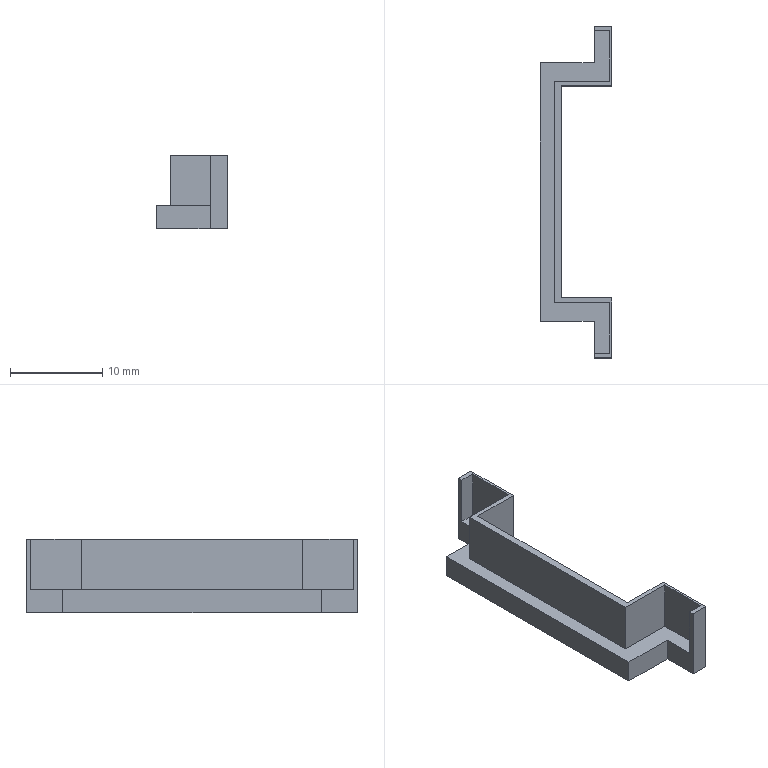Part | STEP file | [DIN35-7.5CA]-1 | 1 solid | 22 faces | box 7.75 x 36 x 8 mm | volume 428.275 mm3 | plane 22
STEP:
#1=CARTESIAN_POINT('',(24.597,-0.5,537.277));
#2=VERTEX_POINT('',#1);
#3=CARTESIAN_POINT('',(24.597,-0.5,539.777));
#4=VERTEX_POINT('',#3);
#5=CARTESIAN_POINT('',(24.597,-0.5,541.277));
#6=DIRECTION('',(0.,0.,1.));
#7=VECTOR('',#6,1000.);
#8=LINE('',#5,#7);
#9=EDGE_CURVE('',#2,#4,#8,.T.);
#10=ORIENTED_EDGE('',*,*,#9,.T.);
#11=CARTESIAN_POINT('',(24.597,27.5,539.777));
#12=VERTEX_POINT('',#11);
#13=CARTESIAN_POINT('',(24.597,-4.,539.777));
#14=DIRECTION('',(0.,1.,0.));
#15=VECTOR('',#14,1000.);
#16=LINE('',#13,#15);
#17=EDGE_CURVE('',#4,#12,#16,.T.);
#18=ORIENTED_EDGE('',*,*,#17,.T.);
#19=CARTESIAN_POINT('',(24.597,27.5,537.277));
#20=VERTEX_POINT('',#19);
#21=CARTESIAN_POINT('',(24.597,27.5,541.277));
#22=DIRECTION('',(0.,0.,-1.));
#23=VECTOR('',#22,1000.);
#24=LINE('',#21,#23);
#25=EDGE_CURVE('',#12,#20,#24,.T.);
#26=ORIENTED_EDGE('',*,*,#25,.T.);
#27=CARTESIAN_POINT('',(24.597,-0.5,537.277));
#28=DIRECTION('',(0.,1.,0.));
#29=VECTOR('',#28,1000.);
#30=LINE('',#27,#29);
#31=EDGE_CURVE('',#2,#20,#30,.T.);
#32=ORIENTED_EDGE('',*,*,#31,.F.);
#33=EDGE_LOOP('',(#10,#18,#26,#32));
#34=FACE_OUTER_BOUND('',#33,.T.);
#35=CARTESIAN_POINT('',(24.597,-0.5,541.277));
#36=DIRECTION('',(-1.,0.,0.));
#37=DIRECTION('',(0.,1.,0.));
#38=AXIS2_PLACEMENT_3D('',#35,#36,#37);
#39=PLANE('',#38);
#40=ADVANCED_FACE('',(#34),#39,.T.);
#41=CARTESIAN_POINT('',(32.347,31.5,545.277));
#42=VERTEX_POINT('',#41);
#43=CARTESIAN_POINT('',(30.447,31.5,545.277));
#44=VERTEX_POINT('',#43);
#45=CARTESIAN_POINT('',(31.397,31.5,545.277));
#46=DIRECTION('',(-1.,0.,0.));
#47=VECTOR('',#46,1000.);
#48=LINE('',#45,#47);
#49=EDGE_CURVE('',#42,#44,#48,.T.);
#50=ORIENTED_EDGE('',*,*,#49,.F.);
#51=CARTESIAN_POINT('',(32.347,31.5,537.277));
#52=VERTEX_POINT('',#51);
#53=CARTESIAN_POINT('',(32.347,31.5,541.277));
#54=DIRECTION('',(0.,0.,1.));
#55=VECTOR('',#54,1000.);
#56=LINE('',#53,#55);
#57=EDGE_CURVE('',#52,#42,#56,.T.);
#58=ORIENTED_EDGE('',*,*,#57,.F.);
#59=CARTESIAN_POINT('',(30.447,31.5,537.277));
#60=VERTEX_POINT('',#59);
#61=CARTESIAN_POINT('',(31.397,31.5,537.277));
#62=DIRECTION('',(1.,0.,0.));
#63=VECTOR('',#62,1000.);
#64=LINE('',#61,#63);
#65=EDGE_CURVE('',#60,#52,#64,.T.);
#66=ORIENTED_EDGE('',*,*,#65,.F.);
#67=CARTESIAN_POINT('',(30.447,31.5,541.277));
#68=DIRECTION('',(0.,0.,-1.));
#69=VECTOR('',#68,1000.);
#70=LINE('',#67,#69);
#71=EDGE_CURVE('',#44,#60,#70,.T.);
#72=ORIENTED_EDGE('',*,*,#71,.F.);
#73=EDGE_LOOP('',(#50,#58,#66,#72));
#74=FACE_OUTER_BOUND('',#73,.T.);
#75=CARTESIAN_POINT('',(31.397,31.5,541.277));
#76=DIRECTION('',(0.,1.,0.));
#77=DIRECTION('',(1.,0.,0.));
#78=AXIS2_PLACEMENT_3D('',#75,#76,#77);
#79=PLANE('',#78);
#80=ADVANCED_FACE('',(#74),#79,.T.);
#81=CARTESIAN_POINT('',(30.447,-4.,545.277));
#82=VERTEX_POINT('',#81);
#83=CARTESIAN_POINT('',(32.097,-4.,545.277));
#84=VERTEX_POINT('',#83);
#85=CARTESIAN_POINT('',(31.347,-4.,545.277));
#86=DIRECTION('',(1.,0.,0.));
#87=VECTOR('',#86,1000.);
#88=LINE('',#85,#87);
#89=EDGE_CURVE('',#82,#84,#88,.T.);
#90=ORIENTED_EDGE('',*,*,#89,.F.);
#91=CARTESIAN_POINT('',(30.447,-4.5,545.277));
#92=VERTEX_POINT('',#91);
#93=CARTESIAN_POINT('',(30.447,-4.5,545.277));
#94=DIRECTION('',(0.,1.,0.));
#95=VECTOR('',#94,1000.);
#96=LINE('',#93,#95);
#97=EDGE_CURVE('',#92,#82,#96,.T.);
#98=ORIENTED_EDGE('',*,*,#97,.F.);
#99=CARTESIAN_POINT('',(32.347,-4.5,545.277));
#100=VERTEX_POINT('',#99);
#101=CARTESIAN_POINT('',(31.397,-4.5,545.277));
#102=DIRECTION('',(1.,0.,0.));
#103=VECTOR('',#102,1000.);
#104=LINE('',#101,#103);
#105=EDGE_CURVE('',#92,#100,#104,.T.);
#106=ORIENTED_EDGE('',*,*,#105,.T.);
#107=CARTESIAN_POINT('',(32.347,2.,545.277));
#108=VERTEX_POINT('',#107);
#109=CARTESIAN_POINT('',(32.347,-4.5,545.277));
#110=DIRECTION('',(0.,1.,0.));
#111=VECTOR('',#110,1000.);
#112=LINE('',#109,#111);
#113=EDGE_CURVE('',#100,#108,#112,.T.);
#114=ORIENTED_EDGE('',*,*,#113,.T.);
#115=CARTESIAN_POINT('',(26.897,2.,545.277));
#116=VERTEX_POINT('',#115);
#117=CARTESIAN_POINT('',(29.622,2.,545.277));
#118=DIRECTION('',(1.,0.,0.));
#119=VECTOR('',#118,1000.);
#120=LINE('',#117,#119);
#121=EDGE_CURVE('',#116,#108,#120,.T.);
#122=ORIENTED_EDGE('',*,*,#121,.F.);
#123=CARTESIAN_POINT('',(26.897,25.,545.277));
#124=VERTEX_POINT('',#123);
#125=CARTESIAN_POINT('',(26.897,2.,545.277));
#126=DIRECTION('',(0.,1.,0.));
#127=VECTOR('',#126,1000.);
#128=LINE('',#125,#127);
#129=EDGE_CURVE('',#116,#124,#128,.T.);
#130=ORIENTED_EDGE('',*,*,#129,.T.);
#131=CARTESIAN_POINT('',(32.347,25.,545.277));
#132=VERTEX_POINT('',#131);
#133=CARTESIAN_POINT('',(29.622,25.,545.277));
#134=DIRECTION('',(-1.,0.,0.));
#135=VECTOR('',#134,1000.);
#136=LINE('',#133,#135);
#137=EDGE_CURVE('',#132,#124,#136,.T.);
#138=ORIENTED_EDGE('',*,*,#137,.F.);
#139=CARTESIAN_POINT('',(32.347,27.5,545.277));
#140=DIRECTION('',(0.,1.,0.));
#141=VECTOR('',#140,1000.);
#142=LINE('',#139,#141);
#143=EDGE_CURVE('',#132,#42,#142,.T.);
#144=ORIENTED_EDGE('',*,*,#143,.T.);
#145=ORIENTED_EDGE('',*,*,#49,.T.);
#146=CARTESIAN_POINT('',(30.447,31.,545.277));
#147=VERTEX_POINT('',#146);
#148=CARTESIAN_POINT('',(30.447,27.5,545.277));
#149=DIRECTION('',(0.,1.,0.));
#150=VECTOR('',#149,1000.);
#151=LINE('',#148,#150);
#152=EDGE_CURVE('',#147,#44,#151,.T.);
#153=ORIENTED_EDGE('',*,*,#152,.F.);
#154=CARTESIAN_POINT('',(32.097,31.,545.277));
#155=VERTEX_POINT('',#154);
#156=CARTESIAN_POINT('',(31.347,31.,545.277));
#157=DIRECTION('',(-1.,0.,0.));
#158=VECTOR('',#157,1000.);
#159=LINE('',#156,#158);
#160=EDGE_CURVE('',#155,#147,#159,.T.);
#161=ORIENTED_EDGE('',*,*,#160,.F.);
#162=CARTESIAN_POINT('',(32.097,25.5,545.277));
#163=VERTEX_POINT('',#162);
#164=CARTESIAN_POINT('',(32.097,27.,545.277));
#165=DIRECTION('',(0.,1.,0.));
#166=VECTOR('',#165,1000.);
#167=LINE('',#164,#166);
#168=EDGE_CURVE('',#163,#155,#167,.T.);
#169=ORIENTED_EDGE('',*,*,#168,.F.);
#170=CARTESIAN_POINT('',(26.097,25.5,545.277));
#171=VERTEX_POINT('',#170);
#172=CARTESIAN_POINT('',(29.097,25.5,545.277));
#173=DIRECTION('',(-1.,0.,0.));
#174=VECTOR('',#173,1000.);
#175=LINE('',#172,#174);
#176=EDGE_CURVE('',#163,#171,#175,.T.);
#177=ORIENTED_EDGE('',*,*,#176,.T.);
#178=CARTESIAN_POINT('',(26.097,1.5,545.277));
#179=VERTEX_POINT('',#178);
#180=CARTESIAN_POINT('',(26.097,1.5,545.277));
#181=DIRECTION('',(0.,1.,0.));
#182=VECTOR('',#181,1000.);
#183=LINE('',#180,#182);
#184=EDGE_CURVE('',#179,#171,#183,.T.);
#185=ORIENTED_EDGE('',*,*,#184,.F.);
#186=CARTESIAN_POINT('',(32.097,1.5,545.277));
#187=VERTEX_POINT('',#186);
#188=CARTESIAN_POINT('',(29.097,1.5,545.277));
#189=DIRECTION('',(1.,0.,0.));
#190=VECTOR('',#189,1000.);
#191=LINE('',#188,#190);
#192=EDGE_CURVE('',#179,#187,#191,.T.);
#193=ORIENTED_EDGE('',*,*,#192,.T.);
#194=CARTESIAN_POINT('',(32.097,-4.,545.277));
#195=DIRECTION('',(0.,1.,0.));
#196=VECTOR('',#195,1000.);
#197=LINE('',#194,#196);
#198=EDGE_CURVE('',#84,#187,#197,.T.);
#199=ORIENTED_EDGE('',*,*,#198,.F.);
#200=EDGE_LOOP('',(#90,#98,#106,#114,#122,#130,#138,#144,#145,#153,#161,#169,#177,#185,#193,#199));
#201=FACE_OUTER_BOUND('',#200,.T.);
#202=CARTESIAN_POINT('',(31.397,27.5,545.277));
#203=DIRECTION('',(0.,0.,1.));
#204=DIRECTION('',(0.,-1.,0.));
#205=AXIS2_PLACEMENT_3D('',#202,#203,#204);
#206=PLANE('',#205);
#207=ADVANCED_FACE('',(#201),#206,.T.);
#208=CARTESIAN_POINT('',(30.447,31.,539.777));
#209=VERTEX_POINT('',#208);
#210=CARTESIAN_POINT('',(30.447,31.,541.277));
#211=DIRECTION('',(0.,0.,-1.));
#212=VECTOR('',#211,1000.);
#213=LINE('',#210,#212);
#214=EDGE_CURVE('',#147,#209,#213,.T.);
#215=ORIENTED_EDGE('',*,*,#214,.F.);
#216=ORIENTED_EDGE('',*,*,#152,.T.);
#217=ORIENTED_EDGE('',*,*,#71,.T.);
#218=CARTESIAN_POINT('',(30.447,27.5,537.277));
#219=VERTEX_POINT('',#218);
#220=CARTESIAN_POINT('',(30.447,27.5,537.277));
#221=DIRECTION('',(0.,1.,0.));
#222=VECTOR('',#221,1000.);
#223=LINE('',#220,#222);
#224=EDGE_CURVE('',#219,#60,#223,.T.);
#225=ORIENTED_EDGE('',*,*,#224,.F.);
#226=CARTESIAN_POINT('',(30.447,27.5,539.777));
#227=VERTEX_POINT('',#226);
#228=CARTESIAN_POINT('',(30.447,27.5,541.277));
#229=DIRECTION('',(0.,0.,1.));
#230=VECTOR('',#229,1000.);
#231=LINE('',#228,#230);
#232=EDGE_CURVE('',#219,#227,#231,.T.);
#233=ORIENTED_EDGE('',*,*,#232,.T.);
#234=CARTESIAN_POINT('',(30.447,27.5,539.777));
#235=DIRECTION('',(0.,-1.,0.));
#236=VECTOR('',#235,1000.);
#237=LINE('',#234,#236);
#238=EDGE_CURVE('',#209,#227,#237,.T.);
#239=ORIENTED_EDGE('',*,*,#238,.F.);
#240=EDGE_LOOP('',(#215,#216,#217,#225,#233,#239));
#241=FACE_OUTER_BOUND('',#240,.T.);
#242=CARTESIAN_POINT('',(30.447,27.5,541.277));
#243=DIRECTION('',(-1.,0.,0.));
#244=DIRECTION('',(0.,1.,0.));
#245=AXIS2_PLACEMENT_3D('',#242,#243,#244);
#246=PLANE('',#245);
#247=ADVANCED_FACE('',(#241),#246,.T.);
#248=ORIENTED_EDGE('',*,*,#224,.T.);
#249=ORIENTED_EDGE('',*,*,#65,.T.);
#250=CARTESIAN_POINT('',(32.347,25.,537.277));
#251=VERTEX_POINT('',#250);
#252=CARTESIAN_POINT('',(32.347,27.5,537.277));
#253=DIRECTION('',(0.,1.,0.));
#254=VECTOR('',#253,1000.);
#255=LINE('',#252,#254);
#256=EDGE_CURVE('',#251,#52,#255,.T.);
#257=ORIENTED_EDGE('',*,*,#256,.F.);
#258=CARTESIAN_POINT('',(26.897,25.,537.277));
#259=VERTEX_POINT('',#258);
#260=CARTESIAN_POINT('',(29.622,25.,537.277));
#261=DIRECTION('',(1.,0.,0.));
#262=VECTOR('',#261,1000.);
#263=LINE('',#260,#262);
#264=EDGE_CURVE('',#259,#251,#263,.T.);
#265=ORIENTED_EDGE('',*,*,#264,.F.);
#266=CARTESIAN_POINT('',(26.897,2.,537.277));
#267=VERTEX_POINT('',#266);
#268=CARTESIAN_POINT('',(26.897,2.,537.277));
#269=DIRECTION('',(0.,1.,0.));
#270=VECTOR('',#269,1000.);
#271=LINE('',#268,#270);
#272=EDGE_CURVE('',#267,#259,#271,.T.);
#273=ORIENTED_EDGE('',*,*,#272,.F.);
#274=CARTESIAN_POINT('',(32.347,2.,537.277));
#275=VERTEX_POINT('',#274);
#276=CARTESIAN_POINT('',(29.622,2.,537.277));
#277=DIRECTION('',(-1.,0.,0.));
#278=VECTOR('',#277,1000.);
#279=LINE('',#276,#278);
#280=EDGE_CURVE('',#275,#267,#279,.T.);
#281=ORIENTED_EDGE('',*,*,#280,.F.);
#282=CARTESIAN_POINT('',(32.347,-4.5,537.277));
#283=VERTEX_POINT('',#282);
#284=CARTESIAN_POINT('',(32.347,-4.5,537.277));
#285=DIRECTION('',(0.,1.,0.));
#286=VECTOR('',#285,1000.);
#287=LINE('',#284,#286);
#288=EDGE_CURVE('',#283,#275,#287,.T.);
#289=ORIENTED_EDGE('',*,*,#288,.F.);
#290=CARTESIAN_POINT('',(30.447,-4.5,537.277));
#291=VERTEX_POINT('',#290);
#292=CARTESIAN_POINT('',(31.397,-4.5,537.277));
#293=DIRECTION('',(-1.,0.,0.));
#294=VECTOR('',#293,1000.);
#295=LINE('',#292,#294);
#296=EDGE_CURVE('',#283,#291,#295,.T.);
#297=ORIENTED_EDGE('',*,*,#296,.T.);
#298=CARTESIAN_POINT('',(30.447,-0.5,537.277));
#299=VERTEX_POINT('',#298);
#300=CARTESIAN_POINT('',(30.447,-4.5,537.277));
#301=DIRECTION('',(0.,1.,0.));
#302=VECTOR('',#301,1000.);
#303=LINE('',#300,#302);
#304=EDGE_CURVE('',#291,#299,#303,.T.);
#305=ORIENTED_EDGE('',*,*,#304,.T.);
#306=CARTESIAN_POINT('',(28.472,-0.5,537.277));
#307=DIRECTION('',(-1.,0.,0.));
#308=VECTOR('',#307,1000.);
#309=LINE('',#306,#308);
#310=EDGE_CURVE('',#299,#2,#309,.T.);
#311=ORIENTED_EDGE('',*,*,#310,.T.);
#312=ORIENTED_EDGE('',*,*,#31,.T.);
#313=CARTESIAN_POINT('',(28.472,27.5,537.277));
#314=DIRECTION('',(1.,0.,0.));
#315=VECTOR('',#314,1000.);
#316=LINE('',#313,#315);
#317=EDGE_CURVE('',#20,#219,#316,.T.);
#318=ORIENTED_EDGE('',*,*,#317,.T.);
#319=EDGE_LOOP('',(#248,#249,#257,#265,#273,#281,#289,#297,#305,#311,#312,#318));
#320=FACE_OUTER_BOUND('',#319,.T.);
#321=CARTESIAN_POINT('',(31.397,27.5,537.277));
#322=DIRECTION('',(0.,0.,-1.));
#323=DIRECTION('',(0.,1.,0.));
#324=AXIS2_PLACEMENT_3D('',#321,#322,#323);
#325=PLANE('',#324);
#326=ADVANCED_FACE('',(#320),#325,.T.);
#327=ORIENTED_EDGE('',*,*,#143,.F.);
#328=CARTESIAN_POINT('',(32.347,25.,541.277));
#329=DIRECTION('',(0.,0.,1.));
#330=VECTOR('',#329,1000.);
#331=LINE('',#328,#330);
#332=EDGE_CURVE('',#251,#132,#331,.T.);
#333=ORIENTED_EDGE('',*,*,#332,.F.);
#334=ORIENTED_EDGE('',*,*,#256,.T.);
#335=ORIENTED_EDGE('',*,*,#57,.T.);
#336=EDGE_LOOP('',(#327,#333,#334,#335));
#337=FACE_OUTER_BOUND('',#336,.T.);
#338=CARTESIAN_POINT('',(32.347,27.5,541.277));
#339=DIRECTION('',(1.,0.,0.));
#340=DIRECTION('',(0.,-1.,0.));
#341=AXIS2_PLACEMENT_3D('',#338,#339,#340);
#342=PLANE('',#341);
#343=ADVANCED_FACE('',(#337),#342,.T.);
#344=CARTESIAN_POINT('',(28.472,27.5,539.777));
#345=DIRECTION('',(-1.,0.,0.));
#346=VECTOR('',#345,1000.);
#347=LINE('',#344,#346);
#348=EDGE_CURVE('',#227,#12,#347,.T.);
#349=ORIENTED_EDGE('',*,*,#348,.F.);
#350=ORIENTED_EDGE('',*,*,#232,.F.);
#351=ORIENTED_EDGE('',*,*,#317,.F.);
#352=ORIENTED_EDGE('',*,*,#25,.F.);
#353=EDGE_LOOP('',(#349,#350,#351,#352));
#354=FACE_OUTER_BOUND('',#353,.T.);
#355=CARTESIAN_POINT('',(28.472,27.5,541.277));
#356=DIRECTION('',(0.,1.,0.));
#357=DIRECTION('',(1.,0.,0.));
#358=AXIS2_PLACEMENT_3D('',#355,#356,#357);
#359=PLANE('',#358);
#360=ADVANCED_FACE('',(#354),#359,.T.);
#361=CARTESIAN_POINT('',(30.447,-0.5,539.777));
#362=VERTEX_POINT('',#361);
#363=CARTESIAN_POINT('',(30.447,-4.,539.777));
#364=VERTEX_POINT('',#363);
#365=CARTESIAN_POINT('',(30.447,-4.5,539.777));
#366=DIRECTION('',(0.,-1.,0.));
#367=VECTOR('',#366,1000.);
#368=LINE('',#365,#367);
#369=EDGE_CURVE('',#362,#364,#368,.T.);
#370=ORIENTED_EDGE('',*,*,#369,.F.);
#371=CARTESIAN_POINT('',(30.447,-0.5,541.277));
#372=DIRECTION('',(0.,0.,-1.));
#373=VECTOR('',#372,1000.);
#374=LINE('',#371,#373);
#375=EDGE_CURVE('',#362,#299,#374,.T.);
#376=ORIENTED_EDGE('',*,*,#375,.T.);
#377=ORIENTED_EDGE('',*,*,#304,.F.);
#378=CARTESIAN_POINT('',(30.447,-4.5,541.277));
#379=DIRECTION('',(0.,0.,1.));
#380=VECTOR('',#379,1000.);
#381=LINE('',#378,#380);
#382=EDGE_CURVE('',#291,#92,#381,.T.);
#383=ORIENTED_EDGE('',*,*,#382,.T.);
#384=ORIENTED_EDGE('',*,*,#97,.T.);
#385=CARTESIAN_POINT('',(30.447,-4.,541.277));
#386=DIRECTION('',(0.,0.,1.));
#387=VECTOR('',#386,1000.);
#388=LINE('',#385,#387);
#389=EDGE_CURVE('',#364,#82,#388,.T.);
#390=ORIENTED_EDGE('',*,*,#389,.F.);
#391=EDGE_LOOP('',(#370,#376,#377,#383,#384,#390));
#392=FACE_OUTER_BOUND('',#391,.T.);
#393=CARTESIAN_POINT('',(30.447,-4.5,541.277));
#394=DIRECTION('',(-1.,0.,0.));
#395=DIRECTION('',(0.,1.,0.));
#396=AXIS2_PLACEMENT_3D('',#393,#394,#395);
#397=PLANE('',#396);
#398=ADVANCED_FACE('',(#392),#397,.T.);
#399=CARTESIAN_POINT('',(32.347,-4.5,541.277));
#400=DIRECTION('',(0.,0.,-1.));
#401=VECTOR('',#400,1000.);
#402=LINE('',#399,#401);
#403=EDGE_CURVE('',#100,#283,#402,.T.);
#404=ORIENTED_EDGE('',*,*,#403,.F.);
#405=ORIENTED_EDGE('',*,*,#105,.F.);
#406=ORIENTED_EDGE('',*,*,#382,.F.);
#407=ORIENTED_EDGE('',*,*,#296,.F.);
#408=EDGE_LOOP('',(#404,#405,#406,#407));
#409=FACE_OUTER_BOUND('',#408,.T.);
#410=CARTESIAN_POINT('',(31.397,-4.5,541.277));
#411=DIRECTION('',(0.,-1.,0.));
#412=DIRECTION('',(-1.,0.,0.));
#413=AXIS2_PLACEMENT_3D('',#410,#411,#412);
#414=PLANE('',#413);
#415=ADVANCED_FACE('',(#409),#414,.T.);
#416=ORIENTED_EDGE('',*,*,#403,.T.);
#417=ORIENTED_EDGE('',*,*,#288,.T.);
#418=CARTESIAN_POINT('',(32.347,2.,541.277));
#419=DIRECTION('',(0.,0.,-1.));
#420=VECTOR('',#419,1000.);
#421=LINE('',#418,#420);
#422=EDGE_CURVE('',#108,#275,#421,.T.);
#423=ORIENTED_EDGE('',*,*,#422,.F.);
#424=ORIENTED_EDGE('',*,*,#113,.F.);
#425=EDGE_LOOP('',(#416,#417,#423,#424));
#426=FACE_OUTER_BOUND('',#425,.T.);
#427=CARTESIAN_POINT('',(32.347,-4.5,541.277));
#428=DIRECTION('',(1.,0.,0.));
#429=DIRECTION('',(0.,-1.,0.));
#430=AXIS2_PLACEMENT_3D('',#427,#428,#429);
#431=PLANE('',#430);
#432=ADVANCED_FACE('',(#426),#431,.T.);
#433=CARTESIAN_POINT('',(28.472,-0.5,539.777));
#434=DIRECTION('',(1.,0.,0.));
#435=VECTOR('',#434,1000.);
#436=LINE('',#433,#435);
#437=EDGE_CURVE('',#4,#362,#436,.T.);
#438=ORIENTED_EDGE('',*,*,#437,.F.);
#439=ORIENTED_EDGE('',*,*,#9,.F.);
#440=ORIENTED_EDGE('',*,*,#310,.F.);
#441=ORIENTED_EDGE('',*,*,#375,.F.);
#442=EDGE_LOOP('',(#438,#439,#440,#441));
#443=FACE_OUTER_BOUND('',#442,.T.);
#444=CARTESIAN_POINT('',(28.472,-0.5,541.277));
#445=DIRECTION('',(0.,-1.,0.));
#446=DIRECTION('',(-1.,0.,0.));
#447=AXIS2_PLACEMENT_3D('',#444,#445,#446);
#448=PLANE('',#447);
#449=ADVANCED_FACE('',(#443),#448,.T.);
#450=ORIENTED_EDGE('',*,*,#137,.T.);
#451=CARTESIAN_POINT('',(26.897,25.,541.277));
#452=DIRECTION('',(0.,0.,-1.));
#453=VECTOR('',#452,1000.);
#454=LINE('',#451,#453);
#455=EDGE_CURVE('',#124,#259,#454,.T.);
#456=ORIENTED_EDGE('',*,*,#455,.T.);
#457=ORIENTED_EDGE('',*,*,#264,.T.);
#458=ORIENTED_EDGE('',*,*,#332,.T.);
#459=EDGE_LOOP('',(#450,#456,#457,#458));
#460=FACE_OUTER_BOUND('',#459,.T.);
#461=CARTESIAN_POINT('',(29.622,25.,541.277));
#462=DIRECTION('',(0.,1.,0.));
#463=DIRECTION('',(1.,0.,0.));
#464=AXIS2_PLACEMENT_3D('',#461,#462,#463);
#465=PLANE('',#464);
#466=ADVANCED_FACE('',(#460),#465,.F.);
#467=ORIENTED_EDGE('',*,*,#129,.F.);
#468=CARTESIAN_POINT('',(26.897,2.,541.277));
#469=DIRECTION('',(0.,0.,1.));
#470=VECTOR('',#469,1000.);
#471=LINE('',#468,#470);
#472=EDGE_CURVE('',#267,#116,#471,.T.);
#473=ORIENTED_EDGE('',*,*,#472,.F.);
#474=ORIENTED_EDGE('',*,*,#272,.T.);
#475=ORIENTED_EDGE('',*,*,#455,.F.);
#476=EDGE_LOOP('',(#467,#473,#474,#475));
#477=FACE_OUTER_BOUND('',#476,.T.);
#478=CARTESIAN_POINT('',(26.897,2.,541.277));
#479=DIRECTION('',(-1.,0.,0.));
#480=DIRECTION('',(0.,1.,0.));
#481=AXIS2_PLACEMENT_3D('',#478,#479,#480);
#482=PLANE('',#481);
#483=ADVANCED_FACE('',(#477),#482,.F.);
#484=ORIENTED_EDGE('',*,*,#422,.T.);
#485=ORIENTED_EDGE('',*,*,#280,.T.);
#486=ORIENTED_EDGE('',*,*,#472,.T.);
#487=ORIENTED_EDGE('',*,*,#121,.T.);
#488=EDGE_LOOP('',(#484,#485,#486,#487));
#489=FACE_OUTER_BOUND('',#488,.T.);
#490=CARTESIAN_POINT('',(29.622,2.,541.277));
#491=DIRECTION('',(0.,-1.,0.));
#492=DIRECTION('',(-1.,0.,0.));
#493=AXIS2_PLACEMENT_3D('',#490,#491,#492);
#494=PLANE('',#493);
#495=ADVANCED_FACE('',(#489),#494,.F.);
#496=ORIENTED_EDGE('',*,*,#214,.T.);
#497=CARTESIAN_POINT('',(32.097,31.,539.777));
#498=VERTEX_POINT('',#497);
#499=CARTESIAN_POINT('',(31.347,31.,539.777));
#500=DIRECTION('',(1.,0.,0.));
#501=VECTOR('',#500,1000.);
#502=LINE('',#499,#501);
#503=EDGE_CURVE('',#209,#498,#502,.T.);
#504=ORIENTED_EDGE('',*,*,#503,.T.);
#505=CARTESIAN_POINT('',(32.097,31.,542.527));
#506=DIRECTION('',(0.,0.,1.));
#507=VECTOR('',#506,1000.);
#508=LINE('',#505,#507);
#509=EDGE_CURVE('',#498,#155,#508,.T.);
#510=ORIENTED_EDGE('',*,*,#509,.T.);
#511=ORIENTED_EDGE('',*,*,#160,.T.);
#512=EDGE_LOOP('',(#496,#504,#510,#511));
#513=FACE_OUTER_BOUND('',#512,.T.);
#514=CARTESIAN_POINT('',(31.347,31.,542.527));
#515=DIRECTION('',(0.,1.,0.));
#516=DIRECTION('',(1.,0.,0.));
#517=AXIS2_PLACEMENT_3D('',#514,#515,#516);
#518=PLANE('',#517);
#519=ADVANCED_FACE('',(#513),#518,.F.);
#520=ORIENTED_EDGE('',*,*,#238,.T.);
#521=ORIENTED_EDGE('',*,*,#348,.T.);
#522=ORIENTED_EDGE('',*,*,#17,.F.);
#523=ORIENTED_EDGE('',*,*,#437,.T.);
#524=ORIENTED_EDGE('',*,*,#369,.T.);
#525=CARTESIAN_POINT('',(32.097,-4.,539.777));
#526=VERTEX_POINT('',#525);
#527=CARTESIAN_POINT('',(28.347,-4.,539.777));
#528=DIRECTION('',(-1.,0.,0.));
#529=VECTOR('',#528,1000.);
#530=LINE('',#527,#529);
#531=EDGE_CURVE('',#526,#364,#530,.T.);
#532=ORIENTED_EDGE('',*,*,#531,.F.);
#533=CARTESIAN_POINT('',(32.097,1.5,539.777));
#534=VERTEX_POINT('',#533);
#535=CARTESIAN_POINT('',(32.097,-4.,539.777));
#536=DIRECTION('',(0.,1.,0.));
#537=VECTOR('',#536,1000.);
#538=LINE('',#535,#537);
#539=EDGE_CURVE('',#526,#534,#538,.T.);
#540=ORIENTED_EDGE('',*,*,#539,.T.);
#541=CARTESIAN_POINT('',(26.097,1.5,539.777));
#542=VERTEX_POINT('',#541);
#543=CARTESIAN_POINT('',(29.097,1.5,539.777));
#544=DIRECTION('',(-1.,0.,0.));
#545=VECTOR('',#544,1000.);
#546=LINE('',#543,#545);
#547=EDGE_CURVE('',#534,#542,#546,.T.);
#548=ORIENTED_EDGE('',*,*,#547,.T.);
#549=CARTESIAN_POINT('',(26.097,25.5,539.777));
#550=VERTEX_POINT('',#549);
#551=CARTESIAN_POINT('',(26.097,1.5,539.777));
#552=DIRECTION('',(0.,1.,0.));
#553=VECTOR('',#552,1000.);
#554=LINE('',#551,#553);
#555=EDGE_CURVE('',#542,#550,#554,.T.);
#556=ORIENTED_EDGE('',*,*,#555,.T.);
#557=CARTESIAN_POINT('',(32.097,25.5,539.777));
#558=VERTEX_POINT('',#557);
#559=CARTESIAN_POINT('',(29.097,25.5,539.777));
#560=DIRECTION('',(1.,0.,0.));
#561=VECTOR('',#560,1000.);
#562=LINE('',#559,#561);
#563=EDGE_CURVE('',#550,#558,#562,.T.);
#564=ORIENTED_EDGE('',*,*,#563,.T.);
#565=CARTESIAN_POINT('',(32.097,27.,539.777));
#566=DIRECTION('',(0.,1.,0.));
#567=VECTOR('',#566,1000.);
#568=LINE('',#565,#567);
#569=EDGE_CURVE('',#558,#498,#568,.T.);
#570=ORIENTED_EDGE('',*,*,#569,.T.);
#571=ORIENTED_EDGE('',*,*,#503,.F.);
#572=EDGE_LOOP('',(#520,#521,#522,#523,#524,#532,#540,#548,#556,#564,#570,#571));
#573=FACE_OUTER_BOUND('',#572,.T.);
#574=CARTESIAN_POINT('',(31.347,27.,539.777));
#575=DIRECTION('',(0.,0.,-1.));
#576=DIRECTION('',(0.,1.,0.));
#577=AXIS2_PLACEMENT_3D('',#574,#575,#576);
#578=PLANE('',#577);
#579=ADVANCED_FACE('',(#573),#578,.F.);
#580=ORIENTED_EDGE('',*,*,#168,.T.);
#581=ORIENTED_EDGE('',*,*,#509,.F.);
#582=ORIENTED_EDGE('',*,*,#569,.F.);
#583=CARTESIAN_POINT('',(32.097,25.5,542.527));
#584=DIRECTION('',(0.,0.,1.));
#585=VECTOR('',#584,1000.);
#586=LINE('',#583,#585);
#587=EDGE_CURVE('',#558,#163,#586,.T.);
#588=ORIENTED_EDGE('',*,*,#587,.T.);
#589=EDGE_LOOP('',(#580,#581,#582,#588));
#590=FACE_OUTER_BOUND('',#589,.T.);
#591=CARTESIAN_POINT('',(32.097,27.,542.527));
#592=DIRECTION('',(1.,0.,0.));
#593=DIRECTION('',(0.,-1.,0.));
#594=AXIS2_PLACEMENT_3D('',#591,#592,#593);
#595=PLANE('',#594);
#596=ADVANCED_FACE('',(#590),#595,.F.);
#597=ORIENTED_EDGE('',*,*,#389,.T.);
#598=ORIENTED_EDGE('',*,*,#89,.T.);
#599=CARTESIAN_POINT('',(32.097,-4.,542.527));
#600=DIRECTION('',(0.,0.,-1.));
#601=VECTOR('',#600,1000.);
#602=LINE('',#599,#601);
#603=EDGE_CURVE('',#84,#526,#602,.T.);
#604=ORIENTED_EDGE('',*,*,#603,.T.);
#605=ORIENTED_EDGE('',*,*,#531,.T.);
#606=EDGE_LOOP('',(#597,#598,#604,#605));
#607=FACE_OUTER_BOUND('',#606,.T.);
#608=CARTESIAN_POINT('',(31.347,-4.,542.527));
#609=DIRECTION('',(0.,-1.,0.));
#610=DIRECTION('',(-1.,0.,0.));
#611=AXIS2_PLACEMENT_3D('',#608,#609,#610);
#612=PLANE('',#611);
#613=ADVANCED_FACE('',(#607),#612,.F.);
#614=ORIENTED_EDGE('',*,*,#603,.F.);
#615=ORIENTED_EDGE('',*,*,#198,.T.);
#616=CARTESIAN_POINT('',(32.097,1.5,542.527));
#617=DIRECTION('',(0.,0.,-1.));
#618=VECTOR('',#617,1000.);
#619=LINE('',#616,#618);
#620=EDGE_CURVE('',#187,#534,#619,.T.);
#621=ORIENTED_EDGE('',*,*,#620,.T.);
#622=ORIENTED_EDGE('',*,*,#539,.F.);
#623=EDGE_LOOP('',(#614,#615,#621,#622));
#624=FACE_OUTER_BOUND('',#623,.T.);
#625=CARTESIAN_POINT('',(32.097,-4.,542.527));
#626=DIRECTION('',(1.,0.,0.));
#627=DIRECTION('',(0.,-1.,0.));
#628=AXIS2_PLACEMENT_3D('',#625,#626,#627);
#629=PLANE('',#628);
#630=ADVANCED_FACE('',(#624),#629,.F.);
#631=ORIENTED_EDGE('',*,*,#176,.F.);
#632=ORIENTED_EDGE('',*,*,#587,.F.);
#633=ORIENTED_EDGE('',*,*,#563,.F.);
#634=CARTESIAN_POINT('',(26.097,25.5,542.527));
#635=DIRECTION('',(0.,0.,-1.));
#636=VECTOR('',#635,1000.);
#637=LINE('',#634,#636);
#638=EDGE_CURVE('',#171,#550,#637,.T.);
#639=ORIENTED_EDGE('',*,*,#638,.F.);
#640=EDGE_LOOP('',(#631,#632,#633,#639));
#641=FACE_OUTER_BOUND('',#640,.T.);
#642=CARTESIAN_POINT('',(29.097,25.5,542.527));
#643=DIRECTION('',(0.,1.,0.));
#644=DIRECTION('',(1.,0.,0.));
#645=AXIS2_PLACEMENT_3D('',#642,#643,#644);
#646=PLANE('',#645);
#647=ADVANCED_FACE('',(#641),#646,.T.);
#648=ORIENTED_EDGE('',*,*,#184,.T.);
#649=ORIENTED_EDGE('',*,*,#638,.T.);
#650=ORIENTED_EDGE('',*,*,#555,.F.);
#651=CARTESIAN_POINT('',(26.097,1.5,542.527));
#652=DIRECTION('',(0.,0.,1.));
#653=VECTOR('',#652,1000.);
#654=LINE('',#651,#653);
#655=EDGE_CURVE('',#542,#179,#654,.T.);
#656=ORIENTED_EDGE('',*,*,#655,.T.);
#657=EDGE_LOOP('',(#648,#649,#650,#656));
#658=FACE_OUTER_BOUND('',#657,.T.);
#659=CARTESIAN_POINT('',(26.097,1.5,542.527));
#660=DIRECTION('',(-1.,0.,0.));
#661=DIRECTION('',(0.,1.,0.));
#662=AXIS2_PLACEMENT_3D('',#659,#660,#661);
#663=PLANE('',#662);
#664=ADVANCED_FACE('',(#658),#663,.T.);
#665=ORIENTED_EDGE('',*,*,#620,.F.);
#666=ORIENTED_EDGE('',*,*,#192,.F.);
#667=ORIENTED_EDGE('',*,*,#655,.F.);
#668=ORIENTED_EDGE('',*,*,#547,.F.);
#669=EDGE_LOOP('',(#665,#666,#667,#668));
#670=FACE_OUTER_BOUND('',#669,.T.);
#671=CARTESIAN_POINT('',(29.097,1.5,542.527));
#672=DIRECTION('',(0.,-1.,0.));
#673=DIRECTION('',(-1.,0.,0.));
#674=AXIS2_PLACEMENT_3D('',#671,#672,#673);
#675=PLANE('',#674);
#676=ADVANCED_FACE('',(#670),#675,.T.);
#677=CLOSED_SHELL('',(#40,#80,#207,#247,#326,#343,#360,#398,#415,#432,#449,#466,#483,#495,#519,#579,#596,#613,#630,#647,#664,#676));
#678=MANIFOLD_SOLID_BREP('',#677);
#679=CARTESIAN_POINT('',(0.,0.,0.));
#680=DIRECTION('',(0.,0.,1.));
#681=DIRECTION('',(1.,0.,0.));
#682=AXIS2_PLACEMENT_3D('',#679,#680,#681);
#683=(LENGTH_UNIT()NAMED_UNIT(*)SI_UNIT(.MILLI.,.METRE.));
#684=UNCERTAINTY_MEASURE_WITH_UNIT(LENGTH_MEASURE(0.00001),#683,'','');
#685=(NAMED_UNIT(*)PLANE_ANGLE_UNIT()SI_UNIT($,.RADIAN.));
#686=(NAMED_UNIT(*)SI_UNIT($,.STERADIAN.)SOLID_ANGLE_UNIT());
#687=(GEOMETRIC_REPRESENTATION_CONTEXT(3)GLOBAL_UNCERTAINTY_ASSIGNED_CONTEXT((#684))GLOBAL_UNIT_ASSIGNED_CONTEXT((#683,#685,#686))REPRESENTATION_CONTEXT('',''));
#688=ADVANCED_BREP_SHAPE_REPRESENTATION('',(#678,#682),#687);